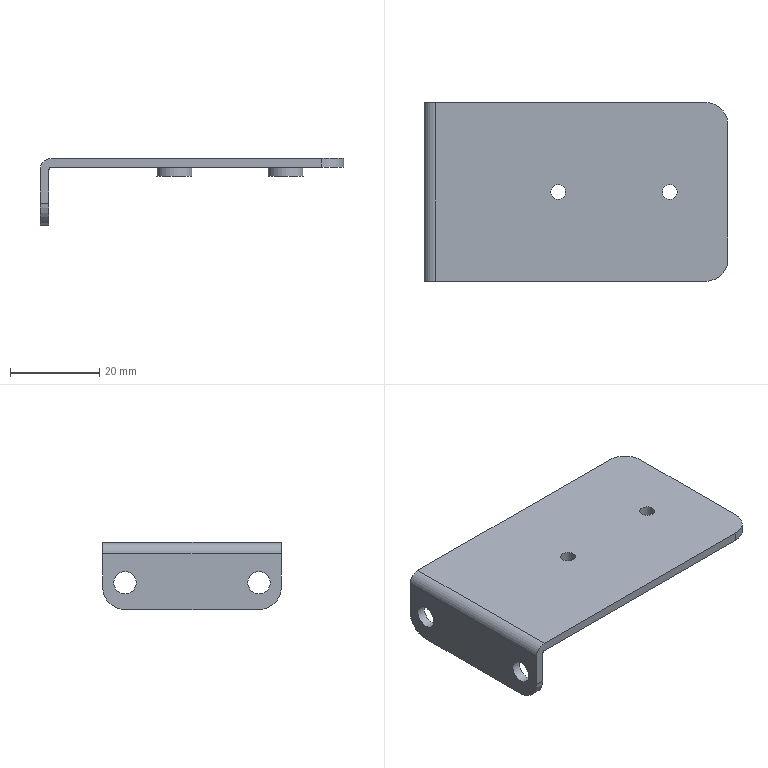Part | STEP file | 1 solid | 22 faces | box 68 x 40 x 15 mm | volume 6435 mm3 | cylinder 12 | plane 10 | commonest cylinder face diameters 10 x4 5 x3 3.3 x2 7.9 x2 1 x1